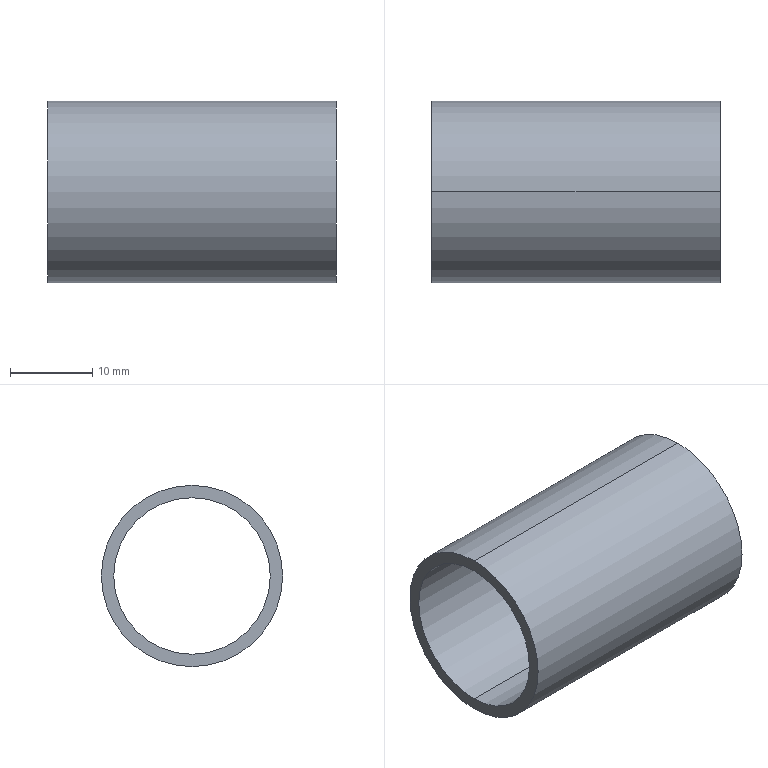Part | STEP file | copper tube 5_default_machined_ | 1 solid | 6 faces | box 35 x 22 x 22 mm | volume 3381 mm3 | cylinder 4 | plane 2 | commonest cylinder face diameters 19 x2 22 x2
STEP:
#1=CARTESIAN_POINT('',(0.,0.,0.));
#2=DIRECTION('',(0.,0.,1.));
#3=DIRECTION('',(1.,0.,0.));
#4=AXIS2_PLACEMENT_3D('',#1,#2,#3);
#5=CARTESIAN_POINT('',(35.,0.,11.));
#6=VERTEX_POINT('',#5);
#7=CARTESIAN_POINT('',(35.,0.,-11.));
#8=VERTEX_POINT('',#7);
#9=CARTESIAN_POINT('',(35.,0.,0.));
#10=DIRECTION('',(-1.,0.,0.));
#11=DIRECTION('',(0.,0.,1.));
#12=AXIS2_PLACEMENT_3D('',#9,#10,#11);
#13=CIRCLE('',#12,11.);
#14=CARTESIAN_POINT('',(35.,0.,0.));
#15=DIRECTION('',(-1.,0.,0.));
#16=DIRECTION('',(0.,0.,1.));
#17=AXIS2_PLACEMENT_3D('',#14,#15,#16);
#18=CYLINDRICAL_SURFACE('',#17,11.);
#19=CARTESIAN_POINT('',(0.,0.));
#20=DIRECTION('',(1.,0.));
#21=VECTOR('',#20,1.);
#22=LINE('',#19,#21);
#23=(GEOMETRIC_REPRESENTATION_CONTEXT(2)PARAMETRIC_REPRESENTATION_CONTEXT()REPRESENTATION_CONTEXT('',''));
#24=DEFINITIONAL_REPRESENTATION('',(#22),#23);
#25=PCURVE('',#18,#24);
#26=CARTESIAN_POINT('',(35.,0.,0.));
#27=DIRECTION('',(1.,0.,0.));
#28=DIRECTION('',(0.,0.,-1.));
#29=AXIS2_PLACEMENT_3D('',#26,#27,#28);
#30=PLANE('',#29);
#31=CARTESIAN_POINT('',(-11.,0.));
#32=CARTESIAN_POINT('',(-11.,19.053));
#33=CARTESIAN_POINT('',(5.5,9.526));
#34=CARTESIAN_POINT('',(22.,0.));
#35=CARTESIAN_POINT('',(5.5,-9.526));
#36=CARTESIAN_POINT('',(-11.,-19.053));
#37=CARTESIAN_POINT('',(-11.,0.));
#38=(BOUNDED_CURVE()B_SPLINE_CURVE(2,(#31,#32,#33,#34,#35,#36,#37),.UNSPECIFIED.,.T.,.F.)B_SPLINE_CURVE_WITH_KNOTS((1,2,2,2,2,1),(-2.094,0.,2.094,4.189,6.283,8.378),.UNSPECIFIED.)CURVE()GEOMETRIC_REPRESENTATION_ITEM()RATIONAL_B_SPLINE_CURVE((1.,0.5,1.,0.5,1.,0.5,1.))REPRESENTATION_ITEM(''));
#39=(GEOMETRIC_REPRESENTATION_CONTEXT(2)PARAMETRIC_REPRESENTATION_CONTEXT()REPRESENTATION_CONTEXT('',''));
#40=DEFINITIONAL_REPRESENTATION('',(#38),#39);
#41=PCURVE('',#30,#40);
#42=SURFACE_CURVE('',#13,(#25,#41),.PCURVE_S1.);
#43=EDGE_CURVE('',#6,#8,#42,.T.);
#44=ORIENTED_EDGE('',*,*,#43,.T.);
#45=CARTESIAN_POINT('',(0.,0.,-11.));
#46=VERTEX_POINT('',#45);
#47=CARTESIAN_POINT('',(35.,0.,-11.));
#48=DIRECTION('',(-1.,0.,0.));
#49=VECTOR('',#48,1.);
#50=LINE('',#47,#49);
#51=CARTESIAN_POINT('',(3.142,0.));
#52=DIRECTION('',(0.,1.));
#53=VECTOR('',#52,1.);
#54=LINE('',#51,#53);
#55=(GEOMETRIC_REPRESENTATION_CONTEXT(2)PARAMETRIC_REPRESENTATION_CONTEXT()REPRESENTATION_CONTEXT('',''));
#56=DEFINITIONAL_REPRESENTATION('',(#54),#55);
#57=PCURVE('',#18,#56);
#58=CARTESIAN_POINT('',(35.,0.,0.));
#59=DIRECTION('',(-1.,0.,0.));
#60=DIRECTION('',(0.,0.,1.));
#61=AXIS2_PLACEMENT_3D('',#58,#59,#60);
#62=CYLINDRICAL_SURFACE('',#61,11.);
#63=CARTESIAN_POINT('',(3.142,0.));
#64=DIRECTION('',(0.,1.));
#65=VECTOR('',#64,1.);
#66=LINE('',#63,#65);
#67=(GEOMETRIC_REPRESENTATION_CONTEXT(2)PARAMETRIC_REPRESENTATION_CONTEXT()REPRESENTATION_CONTEXT('',''));
#68=DEFINITIONAL_REPRESENTATION('',(#66),#67);
#69=PCURVE('',#62,#68);
#70=SURFACE_CURVE('',#50,(#57,#69),.PCURVE_S1.);
#71=EDGE_CURVE('',#8,#46,#70,.T.);
#72=ORIENTED_EDGE('',*,*,#71,.T.);
#73=CARTESIAN_POINT('',(0.,0.,11.));
#74=VERTEX_POINT('',#73);
#75=CARTESIAN_POINT('',(0.,0.,0.));
#76=DIRECTION('',(1.,0.,0.));
#77=DIRECTION('',(0.,0.,1.));
#78=AXIS2_PLACEMENT_3D('',#75,#76,#77);
#79=CIRCLE('',#78,11.);
#80=CARTESIAN_POINT('',(6.283,35.));
#81=DIRECTION('',(-1.,0.));
#82=VECTOR('',#81,1.);
#83=LINE('',#80,#82);
#84=(GEOMETRIC_REPRESENTATION_CONTEXT(2)PARAMETRIC_REPRESENTATION_CONTEXT()REPRESENTATION_CONTEXT('',''));
#85=DEFINITIONAL_REPRESENTATION('',(#83),#84);
#86=PCURVE('',#18,#85);
#87=CARTESIAN_POINT('',(0.,0.,0.));
#88=DIRECTION('',(1.,0.,0.));
#89=DIRECTION('',(0.,0.,-1.));
#90=AXIS2_PLACEMENT_3D('',#87,#88,#89);
#91=PLANE('',#90);
#92=CARTESIAN_POINT('',(0.,0.));
#93=DIRECTION('',(-1.,0.));
#94=AXIS2_PLACEMENT_2D('',#92,#93);
#95=CIRCLE('',#94,11.);
#96=(GEOMETRIC_REPRESENTATION_CONTEXT(2)PARAMETRIC_REPRESENTATION_CONTEXT()REPRESENTATION_CONTEXT('',''));
#97=DEFINITIONAL_REPRESENTATION('',(#95),#96);
#98=PCURVE('',#91,#97);
#99=SURFACE_CURVE('',#79,(#86,#98),.PCURVE_S1.);
#100=EDGE_CURVE('',#46,#74,#99,.T.);
#101=ORIENTED_EDGE('',*,*,#100,.T.);
#102=CARTESIAN_POINT('',(35.,0.,11.));
#103=DIRECTION('',(-1.,0.,0.));
#104=VECTOR('',#103,1.);
#105=LINE('',#102,#104);
#106=CARTESIAN_POINT('',(0.,0.));
#107=DIRECTION('',(0.,1.));
#108=VECTOR('',#107,1.);
#109=LINE('',#106,#108);
#110=(GEOMETRIC_REPRESENTATION_CONTEXT(2)PARAMETRIC_REPRESENTATION_CONTEXT()REPRESENTATION_CONTEXT('',''));
#111=DEFINITIONAL_REPRESENTATION('',(#109),#110);
#112=PCURVE('',#18,#111);
#113=CARTESIAN_POINT('',(6.283,0.));
#114=DIRECTION('',(0.,1.));
#115=VECTOR('',#114,1.);
#116=LINE('',#113,#115);
#117=(GEOMETRIC_REPRESENTATION_CONTEXT(2)PARAMETRIC_REPRESENTATION_CONTEXT()REPRESENTATION_CONTEXT('',''));
#118=DEFINITIONAL_REPRESENTATION('',(#116),#117);
#119=PCURVE('',#62,#118);
#120=SURFACE_CURVE('',#105,(#112,#119),.PCURVE_S1.);
#121=EDGE_CURVE('',#6,#74,#120,.T.);
#122=ORIENTED_EDGE('',*,*,#121,.F.);
#123=EDGE_LOOP('',(#44,#72,#101,#122));
#124=FACE_BOUND('',#123,.T.);
#125=ADVANCED_FACE('',(#124),#18,.T.);
#126=CARTESIAN_POINT('',(35.,0.,9.5));
#127=VERTEX_POINT('',#126);
#128=CARTESIAN_POINT('',(0.,0.,9.5));
#129=VERTEX_POINT('',#128);
#130=CARTESIAN_POINT('',(35.,0.,9.5));
#131=DIRECTION('',(-1.,0.,0.));
#132=VECTOR('',#131,1.);
#133=LINE('',#130,#132);
#134=CARTESIAN_POINT('',(35.,0.,0.));
#135=DIRECTION('',(-1.,0.,0.));
#136=DIRECTION('',(0.,0.,1.));
#137=AXIS2_PLACEMENT_3D('',#134,#135,#136);
#138=CYLINDRICAL_SURFACE('',#137,9.5);
#139=CARTESIAN_POINT('',(6.283,0.));
#140=DIRECTION('',(0.,1.));
#141=VECTOR('',#140,1.);
#142=LINE('',#139,#141);
#143=(GEOMETRIC_REPRESENTATION_CONTEXT(2)PARAMETRIC_REPRESENTATION_CONTEXT()REPRESENTATION_CONTEXT('',''));
#144=DEFINITIONAL_REPRESENTATION('',(#142),#143);
#145=PCURVE('',#138,#144);
#146=CARTESIAN_POINT('',(35.,0.,0.));
#147=DIRECTION('',(-1.,0.,0.));
#148=DIRECTION('',(0.,0.,1.));
#149=AXIS2_PLACEMENT_3D('',#146,#147,#148);
#150=CYLINDRICAL_SURFACE('',#149,9.5);
#151=CARTESIAN_POINT('',(0.,0.));
#152=DIRECTION('',(0.,1.));
#153=VECTOR('',#152,1.);
#154=LINE('',#151,#153);
#155=(GEOMETRIC_REPRESENTATION_CONTEXT(2)PARAMETRIC_REPRESENTATION_CONTEXT()REPRESENTATION_CONTEXT('',''));
#156=DEFINITIONAL_REPRESENTATION('',(#154),#155);
#157=PCURVE('',#150,#156);
#158=SURFACE_CURVE('',#133,(#145,#157),.PCURVE_S1.);
#159=EDGE_CURVE('',#127,#129,#158,.T.);
#160=ORIENTED_EDGE('',*,*,#159,.T.);
#161=CARTESIAN_POINT('',(0.,0.,-9.5));
#162=VERTEX_POINT('',#161);
#163=CARTESIAN_POINT('',(0.,0.,0.));
#164=DIRECTION('',(-1.,0.,0.));
#165=DIRECTION('',(0.,0.,1.));
#166=AXIS2_PLACEMENT_3D('',#163,#164,#165);
#167=CIRCLE('',#166,9.5);
#168=CARTESIAN_POINT('',(0.,35.));
#169=DIRECTION('',(1.,0.));
#170=VECTOR('',#169,1.);
#171=LINE('',#168,#170);
#172=(GEOMETRIC_REPRESENTATION_CONTEXT(2)PARAMETRIC_REPRESENTATION_CONTEXT()REPRESENTATION_CONTEXT('',''));
#173=DEFINITIONAL_REPRESENTATION('',(#171),#172);
#174=PCURVE('',#138,#173);
#175=CARTESIAN_POINT('',(-9.5,0.));
#176=CARTESIAN_POINT('',(-9.5,16.454));
#177=CARTESIAN_POINT('',(4.75,8.227));
#178=CARTESIAN_POINT('',(19.,0.));
#179=CARTESIAN_POINT('',(4.75,-8.227));
#180=CARTESIAN_POINT('',(-9.5,-16.454));
#181=CARTESIAN_POINT('',(-9.5,0.));
#182=(BOUNDED_CURVE()B_SPLINE_CURVE(2,(#175,#176,#177,#178,#179,#180,#181),.UNSPECIFIED.,.T.,.F.)B_SPLINE_CURVE_WITH_KNOTS((1,2,2,2,2,1),(-2.094,0.,2.094,4.189,6.283,8.378),.UNSPECIFIED.)CURVE()GEOMETRIC_REPRESENTATION_ITEM()RATIONAL_B_SPLINE_CURVE((1.,0.5,1.,0.5,1.,0.5,1.))REPRESENTATION_ITEM(''));
#183=(GEOMETRIC_REPRESENTATION_CONTEXT(2)PARAMETRIC_REPRESENTATION_CONTEXT()REPRESENTATION_CONTEXT('',''));
#184=DEFINITIONAL_REPRESENTATION('',(#182),#183);
#185=PCURVE('',#91,#184);
#186=SURFACE_CURVE('',#167,(#174,#185),.PCURVE_S1.);
#187=EDGE_CURVE('',#162,#129,#186,.T.);
#188=ORIENTED_EDGE('',*,*,#187,.F.);
#189=CARTESIAN_POINT('',(35.,0.,-9.5));
#190=VERTEX_POINT('',#189);
#191=CARTESIAN_POINT('',(35.,0.,-9.5));
#192=DIRECTION('',(-1.,0.,0.));
#193=VECTOR('',#192,1.);
#194=LINE('',#191,#193);
#195=CARTESIAN_POINT('',(3.142,0.));
#196=DIRECTION('',(0.,1.));
#197=VECTOR('',#196,1.);
#198=LINE('',#195,#197);
#199=(GEOMETRIC_REPRESENTATION_CONTEXT(2)PARAMETRIC_REPRESENTATION_CONTEXT()REPRESENTATION_CONTEXT('',''));
#200=DEFINITIONAL_REPRESENTATION('',(#198),#199);
#201=PCURVE('',#138,#200);
#202=CARTESIAN_POINT('',(3.142,0.));
#203=DIRECTION('',(0.,1.));
#204=VECTOR('',#203,1.);
#205=LINE('',#202,#204);
#206=(GEOMETRIC_REPRESENTATION_CONTEXT(2)PARAMETRIC_REPRESENTATION_CONTEXT()REPRESENTATION_CONTEXT('',''));
#207=DEFINITIONAL_REPRESENTATION('',(#205),#206);
#208=PCURVE('',#150,#207);
#209=SURFACE_CURVE('',#194,(#201,#208),.PCURVE_S1.);
#210=EDGE_CURVE('',#190,#162,#209,.T.);
#211=ORIENTED_EDGE('',*,*,#210,.F.);
#212=CARTESIAN_POINT('',(35.,0.,0.));
#213=DIRECTION('',(-1.,0.,0.));
#214=DIRECTION('',(0.,0.,1.));
#215=AXIS2_PLACEMENT_3D('',#212,#213,#214);
#216=CIRCLE('',#215,9.5);
#217=CARTESIAN_POINT('',(0.,0.));
#218=DIRECTION('',(1.,0.));
#219=VECTOR('',#218,1.);
#220=LINE('',#217,#219);
#221=(GEOMETRIC_REPRESENTATION_CONTEXT(2)PARAMETRIC_REPRESENTATION_CONTEXT()REPRESENTATION_CONTEXT('',''));
#222=DEFINITIONAL_REPRESENTATION('',(#220),#221);
#223=PCURVE('',#138,#222);
#224=CARTESIAN_POINT('',(-9.5,0.));
#225=CARTESIAN_POINT('',(-9.5,16.454));
#226=CARTESIAN_POINT('',(4.75,8.227));
#227=CARTESIAN_POINT('',(19.,0.));
#228=CARTESIAN_POINT('',(4.75,-8.227));
#229=CARTESIAN_POINT('',(-9.5,-16.454));
#230=CARTESIAN_POINT('',(-9.5,0.));
#231=(BOUNDED_CURVE()B_SPLINE_CURVE(2,(#224,#225,#226,#227,#228,#229,#230),.UNSPECIFIED.,.T.,.F.)B_SPLINE_CURVE_WITH_KNOTS((1,2,2,2,2,1),(-2.094,0.,2.094,4.189,6.283,8.378),.UNSPECIFIED.)CURVE()GEOMETRIC_REPRESENTATION_ITEM()RATIONAL_B_SPLINE_CURVE((1.,0.5,1.,0.5,1.,0.5,1.))REPRESENTATION_ITEM(''));
#232=(GEOMETRIC_REPRESENTATION_CONTEXT(2)PARAMETRIC_REPRESENTATION_CONTEXT()REPRESENTATION_CONTEXT('',''));
#233=DEFINITIONAL_REPRESENTATION('',(#231),#232);
#234=PCURVE('',#30,#233);
#235=SURFACE_CURVE('',#216,(#223,#234),.PCURVE_S1.);
#236=EDGE_CURVE('',#190,#127,#235,.T.);
#237=ORIENTED_EDGE('',*,*,#236,.T.);
#238=EDGE_LOOP('',(#160,#188,#211,#237));
#239=FACE_BOUND('',#238,.F.);
#240=ADVANCED_FACE('',(#239),#138,.F.);
#241=ORIENTED_EDGE('',*,*,#71,.F.);
#242=CARTESIAN_POINT('',(35.,0.,0.));
#243=DIRECTION('',(-1.,0.,0.));
#244=DIRECTION('',(0.,0.,1.));
#245=AXIS2_PLACEMENT_3D('',#242,#243,#244);
#246=CIRCLE('',#245,11.);
#247=CARTESIAN_POINT('',(0.,0.));
#248=DIRECTION('',(1.,0.));
#249=VECTOR('',#248,1.);
#250=LINE('',#247,#249);
#251=(GEOMETRIC_REPRESENTATION_CONTEXT(2)PARAMETRIC_REPRESENTATION_CONTEXT()REPRESENTATION_CONTEXT('',''));
#252=DEFINITIONAL_REPRESENTATION('',(#250),#251);
#253=PCURVE('',#62,#252);
#254=CARTESIAN_POINT('',(-11.,0.));
#255=CARTESIAN_POINT('',(-11.,19.053));
#256=CARTESIAN_POINT('',(5.5,9.526));
#257=CARTESIAN_POINT('',(22.,0.));
#258=CARTESIAN_POINT('',(5.5,-9.526));
#259=CARTESIAN_POINT('',(-11.,-19.053));
#260=CARTESIAN_POINT('',(-11.,0.));
#261=(BOUNDED_CURVE()B_SPLINE_CURVE(2,(#254,#255,#256,#257,#258,#259,#260),.UNSPECIFIED.,.T.,.F.)B_SPLINE_CURVE_WITH_KNOTS((1,2,2,2,2,1),(-2.094,0.,2.094,4.189,6.283,8.378),.UNSPECIFIED.)CURVE()GEOMETRIC_REPRESENTATION_ITEM()RATIONAL_B_SPLINE_CURVE((1.,0.5,1.,0.5,1.,0.5,1.))REPRESENTATION_ITEM(''));
#262=(GEOMETRIC_REPRESENTATION_CONTEXT(2)PARAMETRIC_REPRESENTATION_CONTEXT()REPRESENTATION_CONTEXT('',''));
#263=DEFINITIONAL_REPRESENTATION('',(#261),#262);
#264=PCURVE('',#30,#263);
#265=SURFACE_CURVE('',#246,(#253,#264),.PCURVE_S1.);
#266=EDGE_CURVE('',#8,#6,#265,.T.);
#267=ORIENTED_EDGE('',*,*,#266,.T.);
#268=ORIENTED_EDGE('',*,*,#121,.T.);
#269=CARTESIAN_POINT('',(0.,0.,0.));
#270=DIRECTION('',(1.,0.,0.));
#271=DIRECTION('',(0.,0.,1.));
#272=AXIS2_PLACEMENT_3D('',#269,#270,#271);
#273=CIRCLE('',#272,11.);
#274=CARTESIAN_POINT('',(6.283,35.));
#275=DIRECTION('',(-1.,0.));
#276=VECTOR('',#275,1.);
#277=LINE('',#274,#276);
#278=(GEOMETRIC_REPRESENTATION_CONTEXT(2)PARAMETRIC_REPRESENTATION_CONTEXT()REPRESENTATION_CONTEXT('',''));
#279=DEFINITIONAL_REPRESENTATION('',(#277),#278);
#280=PCURVE('',#62,#279);
#281=CARTESIAN_POINT('',(0.,0.));
#282=DIRECTION('',(-1.,0.));
#283=AXIS2_PLACEMENT_2D('',#281,#282);
#284=CIRCLE('',#283,11.);
#285=(GEOMETRIC_REPRESENTATION_CONTEXT(2)PARAMETRIC_REPRESENTATION_CONTEXT()REPRESENTATION_CONTEXT('',''));
#286=DEFINITIONAL_REPRESENTATION('',(#284),#285);
#287=PCURVE('',#91,#286);
#288=SURFACE_CURVE('',#273,(#280,#287),.PCURVE_S1.);
#289=EDGE_CURVE('',#74,#46,#288,.T.);
#290=ORIENTED_EDGE('',*,*,#289,.T.);
#291=EDGE_LOOP('',(#241,#267,#268,#290));
#292=FACE_BOUND('',#291,.T.);
#293=ADVANCED_FACE('',(#292),#62,.T.);
#294=ORIENTED_EDGE('',*,*,#289,.F.);
#295=ORIENTED_EDGE('',*,*,#100,.F.);
#296=EDGE_LOOP('',(#294,#295));
#297=FACE_BOUND('',#296,.T.);
#298=CARTESIAN_POINT('',(0.,0.,0.));
#299=DIRECTION('',(-1.,0.,0.));
#300=DIRECTION('',(0.,0.,1.));
#301=AXIS2_PLACEMENT_3D('',#298,#299,#300);
#302=CIRCLE('',#301,9.5);
#303=CARTESIAN_POINT('',(-9.5,0.));
#304=CARTESIAN_POINT('',(-9.5,16.454));
#305=CARTESIAN_POINT('',(4.75,8.227));
#306=CARTESIAN_POINT('',(19.,0.));
#307=CARTESIAN_POINT('',(4.75,-8.227));
#308=CARTESIAN_POINT('',(-9.5,-16.454));
#309=CARTESIAN_POINT('',(-9.5,0.));
#310=(BOUNDED_CURVE()B_SPLINE_CURVE(2,(#303,#304,#305,#306,#307,#308,#309),.UNSPECIFIED.,.T.,.F.)B_SPLINE_CURVE_WITH_KNOTS((1,2,2,2,2,1),(-2.094,0.,2.094,4.189,6.283,8.378),.UNSPECIFIED.)CURVE()GEOMETRIC_REPRESENTATION_ITEM()RATIONAL_B_SPLINE_CURVE((1.,0.5,1.,0.5,1.,0.5,1.))REPRESENTATION_ITEM(''));
#311=(GEOMETRIC_REPRESENTATION_CONTEXT(2)PARAMETRIC_REPRESENTATION_CONTEXT()REPRESENTATION_CONTEXT('',''));
#312=DEFINITIONAL_REPRESENTATION('',(#310),#311);
#313=PCURVE('',#91,#312);
#314=CARTESIAN_POINT('',(0.,35.));
#315=DIRECTION('',(1.,0.));
#316=VECTOR('',#315,1.);
#317=LINE('',#314,#316);
#318=(GEOMETRIC_REPRESENTATION_CONTEXT(2)PARAMETRIC_REPRESENTATION_CONTEXT()REPRESENTATION_CONTEXT('',''));
#319=DEFINITIONAL_REPRESENTATION('',(#317),#318);
#320=PCURVE('',#150,#319);
#321=SURFACE_CURVE('',#302,(#313,#320),.PCURVE_S1.);
#322=EDGE_CURVE('',#129,#162,#321,.T.);
#323=ORIENTED_EDGE('',*,*,#322,.F.);
#324=ORIENTED_EDGE('',*,*,#187,.F.);
#325=EDGE_LOOP('',(#323,#324));
#326=FACE_BOUND('',#325,.T.);
#327=ADVANCED_FACE('',(#297,#326),#91,.F.);
#328=ORIENTED_EDGE('',*,*,#43,.F.);
#329=ORIENTED_EDGE('',*,*,#266,.F.);
#330=EDGE_LOOP('',(#328,#329));
#331=FACE_BOUND('',#330,.T.);
#332=CARTESIAN_POINT('',(35.,0.,0.));
#333=DIRECTION('',(-1.,0.,0.));
#334=DIRECTION('',(0.,0.,1.));
#335=AXIS2_PLACEMENT_3D('',#332,#333,#334);
#336=CIRCLE('',#335,9.5);
#337=CARTESIAN_POINT('',(-9.5,0.));
#338=CARTESIAN_POINT('',(-9.5,16.454));
#339=CARTESIAN_POINT('',(4.75,8.227));
#340=CARTESIAN_POINT('',(19.,0.));
#341=CARTESIAN_POINT('',(4.75,-8.227));
#342=CARTESIAN_POINT('',(-9.5,-16.454));
#343=CARTESIAN_POINT('',(-9.5,0.));
#344=(BOUNDED_CURVE()B_SPLINE_CURVE(2,(#337,#338,#339,#340,#341,#342,#343),.UNSPECIFIED.,.T.,.F.)B_SPLINE_CURVE_WITH_KNOTS((1,2,2,2,2,1),(-2.094,0.,2.094,4.189,6.283,8.378),.UNSPECIFIED.)CURVE()GEOMETRIC_REPRESENTATION_ITEM()RATIONAL_B_SPLINE_CURVE((1.,0.5,1.,0.5,1.,0.5,1.))REPRESENTATION_ITEM(''));
#345=(GEOMETRIC_REPRESENTATION_CONTEXT(2)PARAMETRIC_REPRESENTATION_CONTEXT()REPRESENTATION_CONTEXT('',''));
#346=DEFINITIONAL_REPRESENTATION('',(#344),#345);
#347=PCURVE('',#30,#346);
#348=CARTESIAN_POINT('',(0.,0.));
#349=DIRECTION('',(1.,0.));
#350=VECTOR('',#349,1.);
#351=LINE('',#348,#350);
#352=(GEOMETRIC_REPRESENTATION_CONTEXT(2)PARAMETRIC_REPRESENTATION_CONTEXT()REPRESENTATION_CONTEXT('',''));
#353=DEFINITIONAL_REPRESENTATION('',(#351),#352);
#354=PCURVE('',#150,#353);
#355=SURFACE_CURVE('',#336,(#347,#354),.PCURVE_S1.);
#356=EDGE_CURVE('',#127,#190,#355,.T.);
#357=ORIENTED_EDGE('',*,*,#356,.T.);
#358=ORIENTED_EDGE('',*,*,#236,.T.);
#359=EDGE_LOOP('',(#357,#358));
#360=FACE_BOUND('',#359,.T.);
#361=ADVANCED_FACE('',(#331,#360),#30,.T.);
#362=ORIENTED_EDGE('',*,*,#322,.F.);
#363=ORIENTED_EDGE('',*,*,#159,.F.);
#364=ORIENTED_EDGE('',*,*,#356,.T.);
#365=ORIENTED_EDGE('',*,*,#210,.T.);
#366=EDGE_LOOP('',(#362,#363,#364,#365));
#367=FACE_BOUND('',#366,.F.);
#368=ADVANCED_FACE('',(#367),#150,.F.);
#369=CLOSED_SHELL('',(#125,#240,#293,#327,#361,#368));
#370=MANIFOLD_SOLID_BREP('',#369);
#371=(LENGTH_UNIT()NAMED_UNIT(*)SI_UNIT(.MILLI.,.METRE.));
#372=UNCERTAINTY_MEASURE_WITH_UNIT(LENGTH_MEASURE(0.0000001),#371,'','');
#373=(NAMED_UNIT(*)PLANE_ANGLE_UNIT()SI_UNIT($,.RADIAN.));
#374=(NAMED_UNIT(*)SI_UNIT($,.STERADIAN.)SOLID_ANGLE_UNIT());
#375=(GEOMETRIC_REPRESENTATION_CONTEXT(3)GLOBAL_UNCERTAINTY_ASSIGNED_CONTEXT((#372))GLOBAL_UNIT_ASSIGNED_CONTEXT((#371,#373,#374))REPRESENTATION_CONTEXT('',''));
#376=ADVANCED_BREP_SHAPE_REPRESENTATION('',(#4,#370),#375);